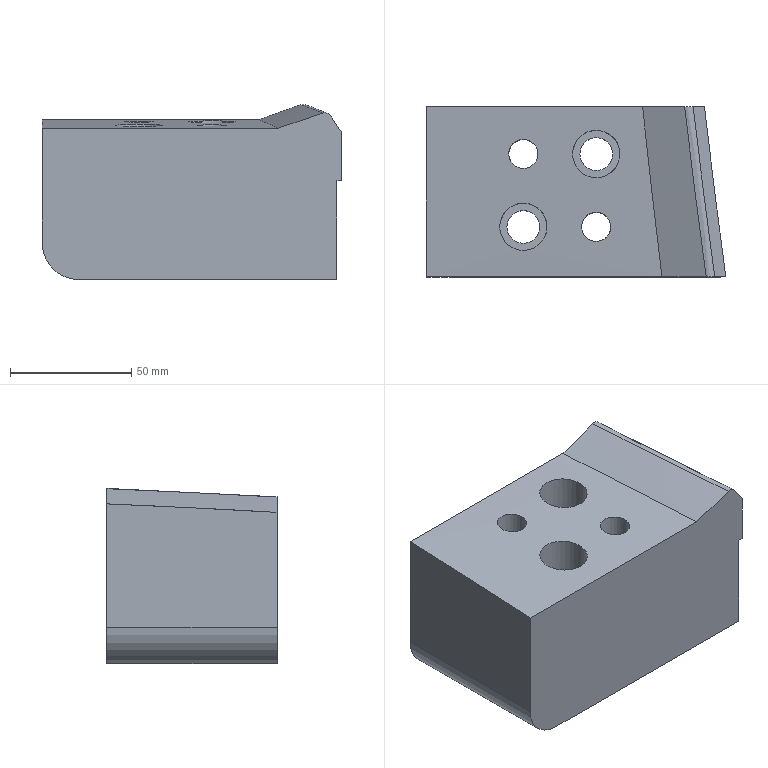Part | NX | features MAIN_BODY 2 | 1 solid | 20 faces | box 123.323 x 70 x 72.141 mm | volume 482943 mm3 | spline 7 | cylinder 7 | plane 6 | commonest cylinder face diameters 12 x2 13.5 x2 19.5 x2 30 x1
STEP:
#1=CARTESIAN_POINT('',(-841.75,-399.358,-100.));
#2=VERTEX_POINT('',#1);
#3=CARTESIAN_POINT('',(-835.,-399.358,-100.));
#4=DIRECTION('',(-0.000000341,0.00000017,-1.));
#5=DIRECTION('',(-1.,0.,0.000000341));
#6=AXIS2_PLACEMENT_3D('',#3,#4,#5);
#7=CIRCLE('',#6,6.75);
#8=EDGE_CURVE('',#2,#2,#7,.T.);
#9=ORIENTED_EDGE('',*,*,#8,.F.);
#10=EDGE_LOOP('',(#9));
#11=FACE_BOUND('',#10,.T.);
#12=CARTESIAN_POINT('',(-841.,-369.358,-100.));
#13=VERTEX_POINT('',#12);
#14=CARTESIAN_POINT('',(-835.,-369.358,-100.));
#15=DIRECTION('',(-0.000000341,0.00000017,-1.));
#16=DIRECTION('',(-1.,0.,0.000000341));
#17=AXIS2_PLACEMENT_3D('',#14,#15,#16);
#18=CIRCLE('',#17,6.);
#19=EDGE_CURVE('',#13,#13,#18,.T.);
#20=ORIENTED_EDGE('',*,*,#19,.F.);
#21=EDGE_LOOP('',(#20));
#22=FACE_BOUND('',#21,.T.);
#23=CARTESIAN_POINT('',(-811.75,-369.358,-100.));
#24=VERTEX_POINT('',#23);
#25=CARTESIAN_POINT('',(-805.,-369.358,-100.));
#26=DIRECTION('',(-0.000000341,0.00000017,-1.));
#27=DIRECTION('',(-1.,0.,0.000000341));
#28=AXIS2_PLACEMENT_3D('',#25,#26,#27);
#29=CIRCLE('',#28,6.75);
#30=EDGE_CURVE('',#24,#24,#29,.T.);
#31=ORIENTED_EDGE('',*,*,#30,.F.);
#32=EDGE_LOOP('',(#31));
#33=FACE_BOUND('',#32,.T.);
#34=CARTESIAN_POINT('',(-811.,-399.358,-100.));
#35=VERTEX_POINT('',#34);
#36=CARTESIAN_POINT('',(-805.,-399.358,-100.));
#37=DIRECTION('',(-0.000000341,0.00000017,-1.));
#38=DIRECTION('',(-1.,0.,0.000000341));
#39=AXIS2_PLACEMENT_3D('',#36,#37,#38);
#40=CIRCLE('',#39,6.);
#41=EDGE_CURVE('',#35,#35,#40,.T.);
#42=ORIENTED_EDGE('',*,*,#41,.F.);
#43=EDGE_LOOP('',(#42));
#44=FACE_BOUND('',#43,.T.);
#45=CARTESIAN_POINT('',(-860.,-350.,-100.));
#46=VERTEX_POINT('',#45);
#47=CARTESIAN_POINT('',(-762.48,-350.,-100.));
#48=VERTEX_POINT('',#47);
#49=CARTESIAN_POINT('',(-0.00003415,-350.,-100.));
#50=DIRECTION('',(-1.,0.,0.000000341));
#51=VECTOR('',#50,1000.);
#52=LINE('',#49,#51);
#53=EDGE_CURVE('',#46,#48,#52,.F.);
#54=ORIENTED_EDGE('',*,*,#53,.T.);
#55=CARTESIAN_POINT('',(-753.694,-420.,-100.));
#56=VERTEX_POINT('',#55);
#57=CARTESIAN_POINT('',(-753.694,-420.,-100.));
#58=CARTESIAN_POINT('',(-755.213,-408.34,-100.));
#59=CARTESIAN_POINT('',(-758.313,-385.028,-100.));
#60=CARTESIAN_POINT('',(-761.09,-361.676,-100.));
#61=CARTESIAN_POINT('',(-762.48,-350.,-100.));
#62=B_SPLINE_CURVE_WITH_KNOTS('',3,(#57,#58,#59,#60,#61),.UNSPECIFIED.,.F.,.F.,(4,1,4),(0.,0.03528,0.07055),.UNSPECIFIED.);
#63=EDGE_CURVE('',#56,#48,#62,.T.);
#64=ORIENTED_EDGE('',*,*,#63,.F.);
#65=CARTESIAN_POINT('',(-860.,-420.,-100.));
#66=VERTEX_POINT('',#65);
#67=CARTESIAN_POINT('',(-0.00003415,-420.,-100.));
#68=DIRECTION('',(-1.,0.,0.000000341));
#69=VECTOR('',#68,1000.);
#70=LINE('',#67,#69);
#71=EDGE_CURVE('',#66,#56,#70,.F.);
#72=ORIENTED_EDGE('',*,*,#71,.F.);
#73=CARTESIAN_POINT('',(-860.,-739.25,-100.));
#74=DIRECTION('',(0.000000011,1.,0.00000017));
#75=VECTOR('',#74,1000.);
#76=LINE('',#73,#75);
#77=EDGE_CURVE('',#46,#66,#76,.F.);
#78=ORIENTED_EDGE('',*,*,#77,.F.);
#79=EDGE_LOOP('',(#54,#64,#72,#78));
#80=FACE_BOUND('',#79,.T.);
#81=CARTESIAN_POINT('',(-780.,-1058.533,-100.));
#82=DIRECTION('',(-0.000000341,0.00000017,-1.));
#83=DIRECTION('',(-0.000000011,-1.,-0.00000017));
#84=AXIS2_PLACEMENT_3D('',#81,#82,#83);
#85=PLANE('',#84);
#86=ADVANCED_FACE('',(#11,#22,#33,#44,#80),#85,.T.);
#87=CARTESIAN_POINT('',(-751.677,-420.,-39.281));
#88=VERTEX_POINT('',#87);
#89=CARTESIAN_POINT('',(-756.237,-420.,-32.638));
#90=VERTEX_POINT('',#89);
#91=CARTESIAN_POINT('',(-751.677,-420.,-39.281));
#92=CARTESIAN_POINT('',(-753.197,-420.,-37.066));
#93=CARTESIAN_POINT('',(-754.717,-420.,-34.852));
#94=CARTESIAN_POINT('',(-756.237,-420.,-32.638));
#95=B_SPLINE_CURVE_WITH_KNOTS('',3,(#91,#92,#93,#94),.UNSPECIFIED.,.F.,.F.,(4,4),(0.,0.008057),.UNSPECIFIED.);
#96=EDGE_CURVE('',#88,#90,#95,.T.);
#97=ORIENTED_EDGE('',*,*,#96,.T.);
#98=CARTESIAN_POINT('',(-759.743,-420.,-31.477));
#99=VERTEX_POINT('',#98);
#100=CARTESIAN_POINT('',(-756.237,-420.,-32.638));
#101=CARTESIAN_POINT('',(-756.992,-420.,-31.539));
#102=CARTESIAN_POINT('',(-758.481,-420.,-31.044));
#103=CARTESIAN_POINT('',(-759.743,-420.,-31.477));
#104=B_SPLINE_CURVE_WITH_KNOTS('',3,(#100,#101,#102,#103),.UNSPECIFIED.,.F.,.F.,(4,4),(0.,0.003944),.UNSPECIFIED.);
#105=EDGE_CURVE('',#90,#99,#104,.T.);
#106=ORIENTED_EDGE('',*,*,#105,.T.);
#107=CARTESIAN_POINT('',(-777.971,-420.,-37.736));
#108=VERTEX_POINT('',#107);
#109=CARTESIAN_POINT('',(-759.743,-420.,-31.477));
#110=CARTESIAN_POINT('',(-765.819,-420.,-33.563));
#111=CARTESIAN_POINT('',(-771.895,-420.,-35.649));
#112=CARTESIAN_POINT('',(-777.971,-420.,-37.736));
#113=B_SPLINE_CURVE_WITH_KNOTS('',3,(#109,#110,#111,#112),.UNSPECIFIED.,.F.,.F.,(4,4),(0.,0.01927),.UNSPECIFIED.);
#114=EDGE_CURVE('',#99,#108,#113,.T.);
#115=ORIENTED_EDGE('',*,*,#114,.T.);
#116=CARTESIAN_POINT('',(-875.,-420.,-37.736));
#117=VERTEX_POINT('',#116);
#118=CARTESIAN_POINT('',(-875.,-420.,-37.736));
#119=CARTESIAN_POINT('',(-842.657,-420.,-37.736));
#120=CARTESIAN_POINT('',(-810.314,-420.,-37.736));
#121=CARTESIAN_POINT('',(-777.971,-420.,-37.736));
#122=B_SPLINE_CURVE_WITH_KNOTS('',3,(#118,#119,#120,#121),.UNSPECIFIED.,.F.,.F.,(4,4),(-0.01,0.08703),.UNSPECIFIED.);
#123=EDGE_CURVE('',#117,#108,#122,.T.);
#124=ORIENTED_EDGE('',*,*,#123,.F.);
#125=CARTESIAN_POINT('',(-875.,-420.,-85.));
#126=VERTEX_POINT('',#125);
#127=CARTESIAN_POINT('',(-875.,-420.,0.0002989));
#128=DIRECTION('',(0.000000341,0.,1.));
#129=VECTOR('',#128,1000.);
#130=LINE('',#127,#129);
#131=EDGE_CURVE('',#126,#117,#130,.T.);
#132=ORIENTED_EDGE('',*,*,#131,.F.);
#133=CARTESIAN_POINT('',(-860.,-420.,-85.));
#134=DIRECTION('',(0.,1.,0.));
#135=DIRECTION('',(0.,0.,1.));
#136=AXIS2_PLACEMENT_3D('',#133,#134,#135);
#137=CIRCLE('',#136,15.);
#138=EDGE_CURVE('',#66,#126,#137,.T.);
#139=ORIENTED_EDGE('',*,*,#138,.F.);
#140=ORIENTED_EDGE('',*,*,#71,.T.);
#141=CARTESIAN_POINT('',(-753.694,-420.,-59.267));
#142=VERTEX_POINT('',#141);
#143=CARTESIAN_POINT('',(-753.694,-420.,-74.594));
#144=DIRECTION('',(0.,0.,1.));
#145=VECTOR('',#144,1000.);
#146=LINE('',#143,#145);
#147=EDGE_CURVE('',#142,#56,#146,.F.);
#148=ORIENTED_EDGE('',*,*,#147,.F.);
#149=CARTESIAN_POINT('',(-751.677,-420.,-59.281));
#150=VERTEX_POINT('',#149);
#151=CARTESIAN_POINT('',(-753.694,-420.,-59.267));
#152=CARTESIAN_POINT('',(-753.022,-420.,-59.272));
#153=CARTESIAN_POINT('',(-752.35,-420.,-59.276));
#154=CARTESIAN_POINT('',(-751.677,-420.,-59.281));
#155=B_SPLINE_CURVE_WITH_KNOTS('',3,(#151,#152,#153,#154),.UNSPECIFIED.,.F.,.F.,(4,4),(0.,0.002017),.UNSPECIFIED.);
#156=EDGE_CURVE('',#142,#150,#155,.T.);
#157=ORIENTED_EDGE('',*,*,#156,.T.);
#158=CARTESIAN_POINT('',(-751.677,-420.,-49.201));
#159=DIRECTION('',(0.,0.,1.));
#160=VECTOR('',#159,1000.);
#161=LINE('',#158,#160);
#162=EDGE_CURVE('',#88,#150,#161,.F.);
#163=ORIENTED_EDGE('',*,*,#162,.F.);
#164=EDGE_LOOP('',(#97,#106,#115,#124,#132,#139,#140,#148,#157,#163));
#165=FACE_BOUND('',#164,.T.);
#166=CARTESIAN_POINT('',(0.,-420.,0.));
#167=DIRECTION('',(0.,1.,0.));
#168=DIRECTION('',(0.,0.,1.));
#169=AXIS2_PLACEMENT_3D('',#166,#167,#168);
#170=PLANE('',#169);
#171=ADVANCED_FACE('',(#165),#170,.F.);
#172=CARTESIAN_POINT('',(-760.466,-350.,-35.75));
#173=VERTEX_POINT('',#172);
#174=CARTESIAN_POINT('',(-760.466,-350.,-55.75));
#175=VERTEX_POINT('',#174);
#176=CARTESIAN_POINT('',(-760.466,-350.,-45.819));
#177=DIRECTION('',(0.,0.,1.));
#178=VECTOR('',#177,1000.);
#179=LINE('',#176,#178);
#180=EDGE_CURVE('',#173,#175,#179,.F.);
#181=ORIENTED_EDGE('',*,*,#180,.F.);
#182=CARTESIAN_POINT('',(-760.466,-350.,-35.75));
#183=CARTESIAN_POINT('',(-759.076,-361.679,-36.278));
#184=CARTESIAN_POINT('',(-756.296,-385.037,-37.348));
#185=CARTESIAN_POINT('',(-753.196,-408.342,-38.648));
#186=CARTESIAN_POINT('',(-751.677,-420.,-39.281));
#187=B_SPLINE_CURVE_WITH_KNOTS('',3,(#182,#183,#184,#185,#186),.UNSPECIFIED.,.F.,.F.,(4,1,4),(-0.001545,0.03377,0.06909),.UNSPECIFIED.);
#188=EDGE_CURVE('',#173,#88,#187,.T.);
#189=ORIENTED_EDGE('',*,*,#188,.T.);
#190=ORIENTED_EDGE('',*,*,#162,.T.);
#191=CARTESIAN_POINT('',(-751.677,-420.,-59.281));
#192=CARTESIAN_POINT('',(-753.196,-408.342,-58.648));
#193=CARTESIAN_POINT('',(-756.296,-385.037,-57.348));
#194=CARTESIAN_POINT('',(-759.076,-361.679,-56.278));
#195=CARTESIAN_POINT('',(-760.466,-350.,-55.75));
#196=B_SPLINE_CURVE_WITH_KNOTS('',3,(#191,#192,#193,#194,#195),.UNSPECIFIED.,.F.,.F.,(4,1,4),(-0.001482,0.03384,0.06916),.UNSPECIFIED.);
#197=EDGE_CURVE('',#150,#175,#196,.T.);
#198=ORIENTED_EDGE('',*,*,#197,.T.);
#199=EDGE_LOOP('',(#181,#189,#190,#198));
#200=FACE_BOUND('',#199,.T.);
#201=CARTESIAN_POINT('',(-760.466,-350.,-55.89));
#202=CARTESIAN_POINT('',(-760.466,-350.,-35.604));
#203=CARTESIAN_POINT('',(-759.076,-361.678,-56.437));
#204=CARTESIAN_POINT('',(-759.076,-361.678,-36.15));
#205=CARTESIAN_POINT('',(-756.296,-385.034,-57.531));
#206=CARTESIAN_POINT('',(-756.296,-385.034,-37.244));
#207=CARTESIAN_POINT('',(-753.196,-408.342,-58.788));
#208=CARTESIAN_POINT('',(-753.196,-408.342,-38.501));
#209=CARTESIAN_POINT('',(-751.677,-420.,-59.401));
#210=CARTESIAN_POINT('',(-751.677,-420.,-39.114));
#211=B_SPLINE_SURFACE_WITH_KNOTS('',3,1,((#201,#202),(#203,#204),(#205,#206),(#207,#208),(#209,#210)),.SURF_OF_LINEAR_EXTRUSION.,.F.,.F.,.F.,(4,1,4),(2,2),(-0.4271,0.68,1.787),(0.,1.),.UNSPECIFIED.);
#212=ADVANCED_FACE('',(#200),#211,.F.);
#213=ORIENTED_EDGE('',*,*,#131,.T.);
#214=CARTESIAN_POINT('',(-875.,-350.,-34.252));
#215=VERTEX_POINT('',#214);
#216=CARTESIAN_POINT('',(-875.,-350.,-34.252));
#217=CARTESIAN_POINT('',(-875.,-373.342,-35.241));
#218=CARTESIAN_POINT('',(-875.,-396.676,-36.394));
#219=CARTESIAN_POINT('',(-875.,-420.,-37.736));
#220=B_SPLINE_CURVE_WITH_KNOTS('',3,(#216,#217,#218,#219),.UNSPECIFIED.,.F.,.F.,(4,4),(0.2837,0.3538),.UNSPECIFIED.);
#221=EDGE_CURVE('',#117,#215,#220,.F.);
#222=ORIENTED_EDGE('',*,*,#221,.T.);
#223=CARTESIAN_POINT('',(-875.,-350.,-85.));
#224=VERTEX_POINT('',#223);
#225=CARTESIAN_POINT('',(-875.,-350.,0.0002989));
#226=DIRECTION('',(0.000000341,0.,1.));
#227=VECTOR('',#226,1000.);
#228=LINE('',#225,#227);
#229=EDGE_CURVE('',#224,#215,#228,.T.);
#230=ORIENTED_EDGE('',*,*,#229,.F.);
#231=CARTESIAN_POINT('',(-875.,-739.25,-85.));
#232=DIRECTION('',(0.000000011,1.,0.00000017));
#233=VECTOR('',#232,1000.);
#234=LINE('',#231,#233);
#235=EDGE_CURVE('',#126,#224,#234,.T.);
#236=ORIENTED_EDGE('',*,*,#235,.F.);
#237=EDGE_LOOP('',(#213,#222,#230,#236));
#238=FACE_BOUND('',#237,.T.);
#239=CARTESIAN_POINT('',(-875.,-739.25,-90.));
#240=DIRECTION('',(-1.,0.000000011,0.000000341));
#241=DIRECTION('',(-0.000000341,0.00000017,-1.));
#242=AXIS2_PLACEMENT_3D('',#239,#240,#241);
#243=PLANE('',#242);
#244=ADVANCED_FACE('',(#238),#243,.T.);
#245=CARTESIAN_POINT('',(-802.615,-378.812,-35.56));
#246=VERTEX_POINT('',#245);
#247=CARTESIAN_POINT('',(-810.554,-378.63,-35.551));
#248=CARTESIAN_POINT('',(-802.353,-379.838,-35.61));
#249=CARTESIAN_POINT('',(-795.722,-374.891,-35.371));
#250=CARTESIAN_POINT('',(-794.523,-366.727,-34.987));
#251=CARTESIAN_POINT('',(-799.45,-360.085,-34.688));
#252=CARTESIAN_POINT('',(-807.643,-358.881,-34.635));
#253=CARTESIAN_POINT('',(-814.27,-363.813,-34.854));
#254=CARTESIAN_POINT('',(-815.479,-371.987,-35.232));
#255=CARTESIAN_POINT('',(-810.554,-378.63,-35.551));
#256=CARTESIAN_POINT('',(-802.353,-379.838,-35.61));
#257=CARTESIAN_POINT('',(-795.722,-374.891,-35.371));
#258=B_SPLINE_CURVE_WITH_KNOTS('',3,(#247,#248,#249,#250,#251,#252,#253,#254,#255,#256,#257),.UNSPECIFIED.,.T.,.F.,(1,1,1,1,1,1,1,1,1,1,1,1,1,1,1),(-0.02287,-0.01525,-0.007624,0.,0.007624,0.01525,0.02287,0.0305,0.03812,0.04574,0.05337,0.06099,0.06862,0.07624,0.08386),.UNSPECIFIED.);
#259=EDGE_CURVE('',#246,#246,#258,.T.);
#260=ORIENTED_EDGE('',*,*,#259,.F.);
#261=EDGE_LOOP('',(#260));
#262=FACE_BOUND('',#261,.T.);
#263=CARTESIAN_POINT('',(-806.104,-405.256,-36.91));
#264=VERTEX_POINT('',#263);
#265=CARTESIAN_POINT('',(-810.492,-403.108,-36.793));
#266=CARTESIAN_POINT('',(-806.223,-405.897,-36.944));
#267=CARTESIAN_POINT('',(-801.239,-404.841,-36.887));
#268=CARTESIAN_POINT('',(-798.467,-400.584,-36.658));
#269=CARTESIAN_POINT('',(-799.51,-395.607,-36.398));
#270=CARTESIAN_POINT('',(-803.775,-392.823,-36.256));
#271=CARTESIAN_POINT('',(-808.753,-393.871,-36.309));
#272=CARTESIAN_POINT('',(-811.534,-398.131,-36.529));
#273=CARTESIAN_POINT('',(-810.492,-403.108,-36.793));
#274=CARTESIAN_POINT('',(-806.223,-405.897,-36.944));
#275=CARTESIAN_POINT('',(-801.239,-404.841,-36.887));
#276=B_SPLINE_CURVE_WITH_KNOTS('',3,(#265,#266,#267,#268,#269,#270,#271,#272,#273,#274,#275),.UNSPECIFIED.,.T.,.F.,(1,1,1,1,1,1,1,1,1,1,1,1,1,1,1),(-0.01408,-0.009385,-0.004692,0.,0.004692,0.009385,0.01408,0.01877,0.02346,0.02815,0.03285,0.03754,0.04223,0.04692,0.05162),.UNSPECIFIED.);
#277=EDGE_CURVE('',#264,#264,#276,.T.);
#278=ORIENTED_EDGE('',*,*,#277,.F.);
#279=EDGE_LOOP('',(#278));
#280=FACE_BOUND('',#279,.T.);
#281=CARTESIAN_POINT('',(-785.933,-350.,-34.252));
#282=VERTEX_POINT('',#281);
#283=CARTESIAN_POINT('',(-875.,-350.,-34.252));
#284=CARTESIAN_POINT('',(-845.311,-350.,-34.252));
#285=CARTESIAN_POINT('',(-815.622,-350.,-34.252));
#286=CARTESIAN_POINT('',(-785.933,-350.,-34.252));
#287=B_SPLINE_CURVE_WITH_KNOTS('',3,(#283,#284,#285,#286),.UNSPECIFIED.,.F.,.F.,(4,4),(-0.01,0.07907),.UNSPECIFIED.);
#288=EDGE_CURVE('',#215,#282,#287,.T.);
#289=ORIENTED_EDGE('',*,*,#288,.F.);
#290=ORIENTED_EDGE('',*,*,#221,.F.);
#291=ORIENTED_EDGE('',*,*,#123,.T.);
#292=CARTESIAN_POINT('',(-777.971,-420.,-37.736));
#293=CARTESIAN_POINT('',(-780.789,-396.695,-36.395));
#294=CARTESIAN_POINT('',(-783.443,-373.36,-35.242));
#295=CARTESIAN_POINT('',(-785.933,-350.,-34.252));
#296=B_SPLINE_CURVE_WITH_KNOTS('',3,(#292,#293,#294,#295),.UNSPECIFIED.,.F.,.F.,(4,4),(0.1656,0.2359),.UNSPECIFIED.);
#297=EDGE_CURVE('',#108,#282,#296,.T.);
#298=ORIENTED_EDGE('',*,*,#297,.T.);
#299=EDGE_LOOP('',(#289,#290,#291,#298));
#300=FACE_BOUND('',#299,.T.);
#301=CARTESIAN_POINT('',(-837.117,-374.973,-35.376));
#302=VERTEX_POINT('',#301);
#303=CARTESIAN_POINT('',(-841.061,-372.092,-35.239));
#304=CARTESIAN_POINT('',(-837.346,-375.582,-35.405));
#305=CARTESIAN_POINT('',(-832.255,-375.414,-35.397));
#306=CARTESIAN_POINT('',(-828.781,-371.706,-35.22));
#307=CARTESIAN_POINT('',(-828.94,-366.622,-34.983));
#308=CARTESIAN_POINT('',(-832.652,-363.137,-34.825));
#309=CARTESIAN_POINT('',(-837.736,-363.299,-34.832));
#310=CARTESIAN_POINT('',(-841.22,-367.009,-35.001));
#311=CARTESIAN_POINT('',(-841.061,-372.092,-35.239));
#312=CARTESIAN_POINT('',(-837.346,-375.582,-35.405));
#313=CARTESIAN_POINT('',(-832.255,-375.414,-35.397));
#314=B_SPLINE_CURVE_WITH_KNOTS('',3,(#303,#304,#305,#306,#307,#308,#309,#310,#311,#312,#313),.UNSPECIFIED.,.T.,.F.,(1,1,1,1,1,1,1,1,1,1,1,1,1,1,1),(-0.01408,-0.009384,-0.004692,0.,0.004692,0.009384,0.01408,0.01877,0.02346,0.02815,0.03284,0.03753,0.04223,0.04692,0.05161),.UNSPECIFIED.);
#315=EDGE_CURVE('',#302,#302,#314,.T.);
#316=ORIENTED_EDGE('',*,*,#315,.F.);
#317=EDGE_LOOP('',(#316));
#318=FACE_BOUND('',#317,.T.);
#319=CARTESIAN_POINT('',(-844.701,-400.333,-36.646));
#320=VERTEX_POINT('',#319);
#321=CARTESIAN_POINT('',(-843.364,-392.516,-36.238));
#322=CARTESIAN_POINT('',(-845.751,-400.44,-36.648));
#323=CARTESIAN_POINT('',(-841.839,-407.721,-37.043));
#324=CARTESIAN_POINT('',(-833.927,-410.11,-37.176));
#325=CARTESIAN_POINT('',(-826.634,-406.198,-36.959));
#326=CARTESIAN_POINT('',(-824.252,-398.282,-36.535));
#327=CARTESIAN_POINT('',(-828.148,-391.005,-36.162));
#328=CARTESIAN_POINT('',(-836.069,-388.604,-36.043));
#329=CARTESIAN_POINT('',(-843.364,-392.516,-36.238));
#330=CARTESIAN_POINT('',(-845.751,-400.44,-36.648));
#331=CARTESIAN_POINT('',(-841.839,-407.721,-37.043));
#332=B_SPLINE_CURVE_WITH_KNOTS('',3,(#321,#322,#323,#324,#325,#326,#327,#328,#329,#330,#331),.UNSPECIFIED.,.T.,.F.,(1,1,1,1,1,1,1,1,1,1,1,1,1,1,1),(-0.02288,-0.01525,-0.007625,0.,0.007625,0.01525,0.02288,0.0305,0.03813,0.04575,0.05338,0.061,0.06863,0.07625,0.08388),.UNSPECIFIED.);
#333=EDGE_CURVE('',#320,#320,#332,.T.);
#334=ORIENTED_EDGE('',*,*,#333,.F.);
#335=EDGE_LOOP('',(#334));
#336=FACE_BOUND('',#335,.T.);
#337=CARTESIAN_POINT('',(-875.566,-420.159,-37.746));
#338=CARTESIAN_POINT('',(-776.547,-420.159,-37.746));
#339=CARTESIAN_POINT('',(-877.1,-408.39,-37.068));
#340=CARTESIAN_POINT('',(-778.081,-408.39,-37.068));
#341=CARTESIAN_POINT('',(-880.224,-384.914,-35.815));
#342=CARTESIAN_POINT('',(-781.205,-384.914,-35.815));
#343=CARTESIAN_POINT('',(-883.011,-361.373,-34.734));
#344=CARTESIAN_POINT('',(-783.992,-361.373,-34.734));
#345=CARTESIAN_POINT('',(-884.415,-349.579,-34.234));
#346=CARTESIAN_POINT('',(-785.396,-349.579,-34.234));
#347=B_SPLINE_SURFACE_WITH_KNOTS('',3,1,((#337,#338),(#339,#340),(#341,#342),(#343,#344),(#345,#346)),.SURF_OF_LINEAR_EXTRUSION.,.F.,.F.,.F.,(4,1,4),(2,2),(-0.0303,0.4972,1.025),(0.,1.),.UNSPECIFIED.);
#348=ADVANCED_FACE('',(#262,#280,#300,#318,#336),#347,.F.);
#349=CARTESIAN_POINT('',(-768.637,-350.,-28.029));
#350=VERTEX_POINT('',#349);
#351=CARTESIAN_POINT('',(-768.637,-350.,-28.029));
#352=CARTESIAN_POINT('',(-774.403,-350.,-30.103));
#353=CARTESIAN_POINT('',(-780.168,-350.,-32.177));
#354=CARTESIAN_POINT('',(-785.933,-350.,-34.252));
#355=B_SPLINE_CURVE_WITH_KNOTS('',3,(#351,#352,#353,#354),.UNSPECIFIED.,.F.,.F.,(4,4),(0.,0.01838),.UNSPECIFIED.);
#356=EDGE_CURVE('',#350,#282,#355,.T.);
#357=ORIENTED_EDGE('',*,*,#356,.F.);
#358=CARTESIAN_POINT('',(-765.126,-350.,-29.138));
#359=VERTEX_POINT('',#358);
#360=CARTESIAN_POINT('',(-768.637,-350.,-28.029));
#361=CARTESIAN_POINT('',(-767.385,-350.,-27.578));
#362=CARTESIAN_POINT('',(-765.892,-350.,-28.05));
#363=CARTESIAN_POINT('',(-765.126,-350.,-29.138));
#364=B_SPLINE_CURVE_WITH_KNOTS('',3,(#360,#361,#362,#363),.UNSPECIFIED.,.F.,.F.,(4,4),(0.,0.003934),.UNSPECIFIED.);
#365=EDGE_CURVE('',#350,#359,#364,.T.);
#366=ORIENTED_EDGE('',*,*,#365,.T.);
#367=CARTESIAN_POINT('',(-765.126,-350.,-29.138));
#368=CARTESIAN_POINT('',(-763.572,-350.,-31.342));
#369=CARTESIAN_POINT('',(-762.019,-350.,-33.546));
#370=CARTESIAN_POINT('',(-760.466,-350.,-35.75));
#371=B_SPLINE_CURVE_WITH_KNOTS('',3,(#367,#368,#369,#370),.UNSPECIFIED.,.F.,.F.,(4,4),(0.,0.008089),.UNSPECIFIED.);
#372=EDGE_CURVE('',#359,#173,#371,.T.);
#373=ORIENTED_EDGE('',*,*,#372,.T.);
#374=ORIENTED_EDGE('',*,*,#180,.T.);
#375=CARTESIAN_POINT('',(-762.48,-350.,-55.739));
#376=VERTEX_POINT('',#375);
#377=CARTESIAN_POINT('',(-760.466,-350.,-55.75));
#378=CARTESIAN_POINT('',(-761.137,-350.,-55.746));
#379=CARTESIAN_POINT('',(-761.808,-350.,-55.743));
#380=CARTESIAN_POINT('',(-762.48,-350.,-55.739));
#381=B_SPLINE_CURVE_WITH_KNOTS('',3,(#377,#378,#379,#380),.UNSPECIFIED.,.F.,.F.,(4,4),(0.,0.002014),.UNSPECIFIED.);
#382=EDGE_CURVE('',#175,#376,#381,.T.);
#383=ORIENTED_EDGE('',*,*,#382,.T.);
#384=CARTESIAN_POINT('',(-762.48,-350.,-72.904));
#385=DIRECTION('',(0.,0.,1.));
#386=VECTOR('',#385,1000.);
#387=LINE('',#384,#386);
#388=EDGE_CURVE('',#376,#48,#387,.F.);
#389=ORIENTED_EDGE('',*,*,#388,.T.);
#390=ORIENTED_EDGE('',*,*,#53,.F.);
#391=CARTESIAN_POINT('',(-860.,-350.,-85.));
#392=DIRECTION('',(0.,1.,0.));
#393=DIRECTION('',(0.,0.,1.));
#394=AXIS2_PLACEMENT_3D('',#391,#392,#393);
#395=CIRCLE('',#394,15.);
#396=EDGE_CURVE('',#224,#46,#395,.F.);
#397=ORIENTED_EDGE('',*,*,#396,.F.);
#398=ORIENTED_EDGE('',*,*,#229,.T.);
#399=ORIENTED_EDGE('',*,*,#288,.T.);
#400=EDGE_LOOP('',(#357,#366,#373,#374,#383,#389,#390,#397,#398,#399));
#401=FACE_BOUND('',#400,.T.);
#402=CARTESIAN_POINT('',(0.,-350.,0.));
#403=DIRECTION('',(0.,1.,0.));
#404=DIRECTION('',(0.,0.,1.));
#405=AXIS2_PLACEMENT_3D('',#402,#403,#404);
#406=PLANE('',#405);
#407=ADVANCED_FACE('',(#401),#406,.T.);
#408=CARTESIAN_POINT('',(-844.75,-399.358,-80.));
#409=VERTEX_POINT('',#408);
#410=CARTESIAN_POINT('',(-835.,-399.358,-80.));
#411=DIRECTION('',(0.000000341,-0.00000017,1.));
#412=DIRECTION('',(-1.,0.,0.000000341));
#413=AXIS2_PLACEMENT_3D('',#410,#411,#412);
#414=CIRCLE('',#413,9.75);
#415=EDGE_CURVE('',#409,#409,#414,.F.);
#416=ORIENTED_EDGE('',*,*,#415,.T.);
#417=EDGE_LOOP('',(#416));
#418=FACE_BOUND('',#417,.T.);
#419=ORIENTED_EDGE('',*,*,#333,.T.);
#420=EDGE_LOOP('',(#419));
#421=FACE_BOUND('',#420,.T.);
#422=CARTESIAN_POINT('',(-835.,-399.358,-70.));
#423=DIRECTION('',(0.000000341,-0.00000017,1.));
#424=DIRECTION('',(0.000000011,1.,0.00000017));
#425=AXIS2_PLACEMENT_3D('',#422,#423,#424);
#426=CYLINDRICAL_SURFACE('',#425,9.75);
#427=ADVANCED_FACE('',(#418,#421),#426,.F.);
#428=CARTESIAN_POINT('',(-841.75,-399.358,-80.));
#429=VERTEX_POINT('',#428);
#430=CARTESIAN_POINT('',(-835.,-399.358,-80.));
#431=DIRECTION('',(0.000000341,-0.00000017,1.));
#432=DIRECTION('',(-1.,0.,0.000000341));
#433=AXIS2_PLACEMENT_3D('',#430,#431,#432);
#434=CIRCLE('',#433,6.75);
#435=EDGE_CURVE('',#429,#429,#434,.F.);
#436=ORIENTED_EDGE('',*,*,#435,.F.);
#437=EDGE_LOOP('',(#436));
#438=FACE_BOUND('',#437,.T.);
#439=ORIENTED_EDGE('',*,*,#8,.T.);
#440=EDGE_LOOP('',(#439));
#441=FACE_BOUND('',#440,.T.);
#442=CARTESIAN_POINT('',(-835.,-399.358,-90.));
#443=DIRECTION('',(0.000000341,-0.00000017,1.));
#444=DIRECTION('',(0.000000011,1.,0.00000017));
#445=AXIS2_PLACEMENT_3D('',#442,#443,#444);
#446=CYLINDRICAL_SURFACE('',#445,6.75);
#447=ADVANCED_FACE('',(#438,#441),#446,.F.);
#448=ORIENTED_EDGE('',*,*,#435,.T.);
#449=EDGE_LOOP('',(#448));
#450=FACE_BOUND('',#449,.T.);
#451=ORIENTED_EDGE('',*,*,#415,.F.);
#452=EDGE_LOOP('',(#451));
#453=FACE_BOUND('',#452,.T.);
#454=CARTESIAN_POINT('',(-835.,-399.358,-80.));
#455=DIRECTION('',(-0.000000341,0.00000017,-1.));
#456=DIRECTION('',(-0.000000011,-1.,-0.00000017));
#457=AXIS2_PLACEMENT_3D('',#454,#455,#456);
#458=PLANE('',#457);
#459=ADVANCED_FACE('',(#450,#453),#458,.F.);
#460=ORIENTED_EDGE('',*,*,#19,.T.);
#461=EDGE_LOOP('',(#460));
#462=FACE_BOUND('',#461,.T.);
#463=ORIENTED_EDGE('',*,*,#315,.T.);
#464=EDGE_LOOP('',(#463));
#465=FACE_BOUND('',#464,.T.);
#466=CARTESIAN_POINT('',(-835.,-369.358,-90.));
#467=DIRECTION('',(0.000000341,-0.00000017,1.));
#468=DIRECTION('',(0.000000011,1.,0.00000017));
#469=AXIS2_PLACEMENT_3D('',#466,#467,#468);
#470=CYLINDRICAL_SURFACE('',#469,6.);
#471=ADVANCED_FACE('',(#462,#465),#470,.F.);
#472=CARTESIAN_POINT('',(-814.75,-369.358,-80.));
#473=VERTEX_POINT('',#472);
#474=CARTESIAN_POINT('',(-805.,-369.358,-80.));
#475=DIRECTION('',(0.000000341,-0.00000017,1.));
#476=DIRECTION('',(-1.,0.,0.000000341));
#477=AXIS2_PLACEMENT_3D('',#474,#475,#476);
#478=CIRCLE('',#477,9.75);
#479=EDGE_CURVE('',#473,#473,#478,.F.);
#480=ORIENTED_EDGE('',*,*,#479,.T.);
#481=EDGE_LOOP('',(#480));
#482=FACE_BOUND('',#481,.T.);
#483=ORIENTED_EDGE('',*,*,#259,.T.);
#484=EDGE_LOOP('',(#483));
#485=FACE_BOUND('',#484,.T.);
#486=CARTESIAN_POINT('',(-805.,-369.358,-70.));
#487=DIRECTION('',(0.000000341,-0.00000017,1.));
#488=DIRECTION('',(0.000000011,1.,0.00000017));
#489=AXIS2_PLACEMENT_3D('',#486,#487,#488);
#490=CYLINDRICAL_SURFACE('',#489,9.75);
#491=ADVANCED_FACE('',(#482,#485),#490,.F.);
#492=CARTESIAN_POINT('',(-811.75,-369.358,-80.));
#493=VERTEX_POINT('',#492);
#494=CARTESIAN_POINT('',(-805.,-369.358,-80.));
#495=DIRECTION('',(0.000000341,-0.00000017,1.));
#496=DIRECTION('',(-1.,0.,0.000000341));
#497=AXIS2_PLACEMENT_3D('',#494,#495,#496);
#498=CIRCLE('',#497,6.75);
#499=EDGE_CURVE('',#493,#493,#498,.F.);
#500=ORIENTED_EDGE('',*,*,#499,.F.);
#501=EDGE_LOOP('',(#500));
#502=FACE_BOUND('',#501,.T.);
#503=ORIENTED_EDGE('',*,*,#30,.T.);
#504=EDGE_LOOP('',(#503));
#505=FACE_BOUND('',#504,.T.);
#506=CARTESIAN_POINT('',(-805.,-369.358,-90.));
#507=DIRECTION('',(0.000000341,-0.00000017,1.));
#508=DIRECTION('',(0.000000011,1.,0.00000017));
#509=AXIS2_PLACEMENT_3D('',#506,#507,#508);
#510=CYLINDRICAL_SURFACE('',#509,6.75);
#511=ADVANCED_FACE('',(#502,#505),#510,.F.);
#512=ORIENTED_EDGE('',*,*,#499,.T.);
#513=EDGE_LOOP('',(#512));
#514=FACE_BOUND('',#513,.T.);
#515=ORIENTED_EDGE('',*,*,#479,.F.);
#516=EDGE_LOOP('',(#515));
#517=FACE_BOUND('',#516,.T.);
#518=CARTESIAN_POINT('',(-805.,-369.358,-80.));
#519=DIRECTION('',(-0.000000341,0.00000017,-1.));
#520=DIRECTION('',(-0.000000011,-1.,-0.00000017));
#521=AXIS2_PLACEMENT_3D('',#518,#519,#520);
#522=PLANE('',#521);
#523=ADVANCED_FACE('',(#514,#517),#522,.F.);
#524=ORIENTED_EDGE('',*,*,#41,.T.);
#525=EDGE_LOOP('',(#524));
#526=FACE_BOUND('',#525,.T.);
#527=ORIENTED_EDGE('',*,*,#277,.T.);
#528=EDGE_LOOP('',(#527));
#529=FACE_BOUND('',#528,.T.);
#530=CARTESIAN_POINT('',(-805.,-399.358,-90.));
#531=DIRECTION('',(0.000000341,-0.00000017,1.));
#532=DIRECTION('',(0.000000011,1.,0.00000017));
#533=AXIS2_PLACEMENT_3D('',#530,#531,#532);
#534=CYLINDRICAL_SURFACE('',#533,6.);
#535=ADVANCED_FACE('',(#526,#529),#534,.F.);
#536=ORIENTED_EDGE('',*,*,#156,.F.);
#537=CARTESIAN_POINT('',(-753.694,-420.,-59.267));
#538=CARTESIAN_POINT('',(-755.213,-408.342,-58.634));
#539=CARTESIAN_POINT('',(-758.312,-385.037,-57.335));
#540=CARTESIAN_POINT('',(-761.09,-361.679,-56.267));
#541=CARTESIAN_POINT('',(-762.48,-350.,-55.739));
#542=B_SPLINE_CURVE_WITH_KNOTS('',3,(#537,#538,#539,#540,#541),.UNSPECIFIED.,.F.,.F.,(4,1,4),(-0.001482,0.03384,0.06916),.UNSPECIFIED.);
#543=EDGE_CURVE('',#142,#376,#542,.T.);
#544=ORIENTED_EDGE('',*,*,#543,.T.);
#545=ORIENTED_EDGE('',*,*,#382,.F.);
#546=ORIENTED_EDGE('',*,*,#197,.F.);
#547=EDGE_LOOP('',(#536,#544,#545,#546));
#548=FACE_BOUND('',#547,.T.);
#549=CARTESIAN_POINT('',(-751.658,-419.997,-59.281));
#550=CARTESIAN_POINT('',(-751.721,-419.508,-59.254));
#551=CARTESIAN_POINT('',(-751.785,-419.019,-59.228));
#552=CARTESIAN_POINT('',(-751.849,-418.53,-59.201));
#553=CARTESIAN_POINT('',(-753.303,-407.372,-58.596));
#554=CARTESIAN_POINT('',(-754.778,-396.218,-57.973));
#555=CARTESIAN_POINT('',(-757.606,-373.887,-56.841));
#556=CARTESIAN_POINT('',(-758.933,-362.709,-56.325));
#557=CARTESIAN_POINT('',(-760.264,-351.53,-55.819));
#558=CARTESIAN_POINT('',(-760.29,-351.307,-55.809));
#559=CARTESIAN_POINT('',(-760.317,-351.083,-55.799));
#560=CARTESIAN_POINT('',(-760.343,-350.86,-55.789));
#561=CARTESIAN_POINT('',(-760.387,-350.493,-55.772));
#562=CARTESIAN_POINT('',(-760.431,-350.127,-55.756));
#563=CARTESIAN_POINT('',(-760.474,-349.761,-55.739));
#564=CARTESIAN_POINT('',(-753.678,-420.261,-59.281));
#565=CARTESIAN_POINT('',(-753.742,-419.771,-59.254));
#566=CARTESIAN_POINT('',(-753.806,-419.282,-59.228));
#567=CARTESIAN_POINT('',(-753.869,-418.793,-59.201));
#568=CARTESIAN_POINT('',(-755.323,-407.637,-58.596));
#569=CARTESIAN_POINT('',(-756.799,-396.482,-57.973));
#570=CARTESIAN_POINT('',(-759.629,-374.135,-56.841));
#571=CARTESIAN_POINT('',(-760.957,-362.946,-56.325));
#572=CARTESIAN_POINT('',(-762.287,-351.771,-55.819));
#573=CARTESIAN_POINT('',(-762.313,-351.548,-55.809));
#574=CARTESIAN_POINT('',(-762.34,-351.324,-55.799));
#575=CARTESIAN_POINT('',(-762.367,-351.101,-55.789));
#576=CARTESIAN_POINT('',(-762.41,-350.734,-55.772));
#577=CARTESIAN_POINT('',(-762.454,-350.368,-55.756));
#578=CARTESIAN_POINT('',(-762.497,-350.002,-55.739));
#579=B_SPLINE_SURFACE_WITH_KNOTS('',1,3,((#549,#550,#551,#552,#553,#554,#555,#556,#557,#558,#559,#560,#561,#562,#563),(#564,#565,#566,#567,#568,#569,#570,#571,#572,#573,#574,#575,#576,#577,#578)),.RULED_SURF.,.F.,.F.,.F.,(2,2),(4,3,2,3,3,4),(0.498,0.7018),(-0.02192,0.,0.5,1.,1.01,1.026),.UNSPECIFIED.);
#580=ADVANCED_FACE('',(#548),#579,.T.);
#581=ORIENTED_EDGE('',*,*,#543,.F.);
#582=ORIENTED_EDGE('',*,*,#147,.T.);
#583=ORIENTED_EDGE('',*,*,#63,.T.);
#584=ORIENTED_EDGE('',*,*,#388,.F.);
#585=EDGE_LOOP('',(#581,#582,#583,#584));
#586=FACE_BOUND('',#585,.T.);
#587=CARTESIAN_POINT('',(-762.48,-350.,-100.266));
#588=CARTESIAN_POINT('',(-762.48,-350.,-55.446));
#589=CARTESIAN_POINT('',(-761.09,-361.674,-100.812));
#590=CARTESIAN_POINT('',(-761.09,-361.674,-55.993));
#591=CARTESIAN_POINT('',(-758.311,-385.042,-101.904));
#592=CARTESIAN_POINT('',(-758.311,-385.042,-57.085));
#593=CARTESIAN_POINT('',(-755.213,-408.345,-103.161));
#594=CARTESIAN_POINT('',(-755.213,-408.345,-58.342));
#595=CARTESIAN_POINT('',(-753.694,-420.,-103.774));
#596=CARTESIAN_POINT('',(-753.694,-420.,-58.954));
#597=B_SPLINE_SURFACE_WITH_KNOTS('',3,1,((#587,#588),(#589,#590),(#591,#592),(#593,#594),(#595,#596)),.SURF_OF_LINEAR_EXTRUSION.,.F.,.F.,.F.,(4,1,4),(2,2),(-0.4346,0.6722,1.779),(0.,1.),.UNSPECIFIED.);
#598=ADVANCED_FACE('',(#586),#597,.F.);
#599=ORIENTED_EDGE('',*,*,#138,.T.);
#600=ORIENTED_EDGE('',*,*,#235,.T.);
#601=ORIENTED_EDGE('',*,*,#396,.T.);
#602=ORIENTED_EDGE('',*,*,#77,.T.);
#603=EDGE_LOOP('',(#599,#600,#601,#602));
#604=FACE_BOUND('',#603,.T.);
#605=CARTESIAN_POINT('',(-860.,-739.25,-85.));
#606=DIRECTION('',(0.000000011,1.,0.00000017));
#607=DIRECTION('',(-0.000000341,0.00000017,-1.));
#608=AXIS2_PLACEMENT_3D('',#605,#606,#607);
#609=CYLINDRICAL_SURFACE('',#608,15.);
#610=ADVANCED_FACE('',(#604),#609,.T.);
#611=ORIENTED_EDGE('',*,*,#114,.F.);
#612=CARTESIAN_POINT('',(-759.743,-420.,-31.477));
#613=CARTESIAN_POINT('',(-762.888,-396.7,-30.139));
#614=CARTESIAN_POINT('',(-765.861,-373.365,-29.002));
#615=CARTESIAN_POINT('',(-768.637,-350.,-28.029));
#616=B_SPLINE_CURVE_WITH_KNOTS('',3,(#612,#613,#614,#615),.UNSPECIFIED.,.F.,.F.,(4,4),(-0.001483,0.06917),.UNSPECIFIED.);
#617=EDGE_CURVE('',#99,#350,#616,.T.);
#618=ORIENTED_EDGE('',*,*,#617,.T.);
#619=ORIENTED_EDGE('',*,*,#356,.T.);
#620=ORIENTED_EDGE('',*,*,#297,.F.);
#621=EDGE_LOOP('',(#611,#618,#619,#620));
#622=FACE_BOUND('',#621,.T.);
#623=CARTESIAN_POINT('',(-786.407,-349.588,-34.389));
#624=CARTESIAN_POINT('',(-780.371,-349.42,-32.203));
#625=CARTESIAN_POINT('',(-774.335,-349.252,-30.016));
#626=CARTESIAN_POINT('',(-768.299,-349.083,-27.83));
#627=CARTESIAN_POINT('',(-783.865,-373.411,-35.389));
#628=CARTESIAN_POINT('',(-777.801,-373.256,-33.222));
#629=CARTESIAN_POINT('',(-771.737,-373.101,-31.056));
#630=CARTESIAN_POINT('',(-765.672,-372.946,-28.89));
#631=CARTESIAN_POINT('',(-781.057,-397.131,-36.53));
#632=CARTESIAN_POINT('',(-774.96,-396.996,-34.387));
#633=CARTESIAN_POINT('',(-768.862,-396.86,-32.244));
#634=CARTESIAN_POINT('',(-762.765,-396.725,-30.101));
#635=CARTESIAN_POINT('',(-777.983,-420.75,-37.815));
#636=CARTESIAN_POINT('',(-771.848,-420.64,-35.698));
#637=CARTESIAN_POINT('',(-765.712,-420.53,-33.581));
#638=CARTESIAN_POINT('',(-759.577,-420.419,-31.464));
#639=B_SPLINE_SURFACE_WITH_KNOTS('',3,3,((#623,#624,#625,#626),(#627,#628,#629,#630),(#631,#632,#633,#634),(#635,#636,#637,#638)),.UNSPECIFIED.,.F.,.F.,.F.,(4,4),(4,4),(0.607,0.7329),(-0.6403,-0.1096),.UNSPECIFIED.);
#640=ADVANCED_FACE('',(#622),#639,.T.);
#641=ORIENTED_EDGE('',*,*,#372,.F.);
#642=CARTESIAN_POINT('',(-765.126,-350.,-29.138));
#643=CARTESIAN_POINT('',(-762.352,-373.365,-30.128));
#644=CARTESIAN_POINT('',(-759.378,-396.7,-31.282));
#645=CARTESIAN_POINT('',(-756.237,-420.,-32.638));
#646=B_SPLINE_CURVE_WITH_KNOTS('',3,(#642,#643,#644,#645),.UNSPECIFIED.,.F.,.F.,(4,4),(-0.001545,0.06911),.UNSPECIFIED.);
#647=EDGE_CURVE('',#359,#90,#646,.T.);
#648=ORIENTED_EDGE('',*,*,#647,.T.);
#649=ORIENTED_EDGE('',*,*,#96,.F.);
#650=ORIENTED_EDGE('',*,*,#188,.F.);
#651=EDGE_LOOP('',(#641,#648,#649,#650));
#652=FACE_BOUND('',#651,.T.);
#653=CARTESIAN_POINT('',(-740.602,-417.938,-55.704));
#654=CARTESIAN_POINT('',(-753.885,-420.924,-35.937));
#655=CARTESIAN_POINT('',(-760.317,-422.37,-26.365));
#656=CARTESIAN_POINT('',(-740.639,-417.646,-55.688));
#657=CARTESIAN_POINT('',(-753.923,-420.629,-35.922));
#658=CARTESIAN_POINT('',(-760.356,-422.074,-26.351));
#659=CARTESIAN_POINT('',(-740.676,-417.353,-55.673));
#660=CARTESIAN_POINT('',(-753.961,-420.334,-35.907));
#661=CARTESIAN_POINT('',(-760.395,-421.778,-26.336));
#662=CARTESIAN_POINT('',(-740.712,-417.061,-55.657));
#663=CARTESIAN_POINT('',(-754.,-420.039,-35.892));
#664=CARTESIAN_POINT('',(-760.433,-421.482,-26.321));
#665=CARTESIAN_POINT('',(-740.749,-416.768,-55.641));
#666=CARTESIAN_POINT('',(-754.038,-419.745,-35.877));
#667=CARTESIAN_POINT('',(-760.472,-421.186,-26.306));
#668=CARTESIAN_POINT('',(-740.786,-416.476,-55.625));
#669=CARTESIAN_POINT('',(-754.076,-419.45,-35.862));
#670=CARTESIAN_POINT('',(-760.511,-420.89,-26.291));
#671=CARTESIAN_POINT('',(-741.502,-410.76,-55.318));
#672=CARTESIAN_POINT('',(-754.82,-413.687,-35.566));
#673=CARTESIAN_POINT('',(-761.268,-415.105,-26.002));
#674=CARTESIAN_POINT('',(-742.219,-405.044,-55.01));
#675=CARTESIAN_POINT('',(-755.564,-407.925,-35.271));
#676=CARTESIAN_POINT('',(-762.026,-409.321,-25.713));
#677=CARTESIAN_POINT('',(-742.935,-399.328,-54.703));
#678=CARTESIAN_POINT('',(-756.308,-402.163,-34.976));
#679=CARTESIAN_POINT('',(-762.783,-403.536,-25.424));
#680=CARTESIAN_POINT('',(-743.651,-393.612,-54.395));
#681=CARTESIAN_POINT('',(-757.052,-396.401,-34.681));
#682=CARTESIAN_POINT('',(-763.54,-397.751,-25.135));
#683=CARTESIAN_POINT('',(-744.368,-387.896,-54.088));
#684=CARTESIAN_POINT('',(-757.796,-390.639,-34.386));
#685=CARTESIAN_POINT('',(-764.298,-391.967,-24.846));
#686=CARTESIAN_POINT('',(-744.908,-383.586,-53.856));
#687=CARTESIAN_POINT('',(-758.357,-386.294,-34.163));
#688=CARTESIAN_POINT('',(-764.869,-387.605,-24.628));
#689=CARTESIAN_POINT('',(-745.44,-379.274,-53.629));
#690=CARTESIAN_POINT('',(-758.909,-381.948,-33.945));
#691=CARTESIAN_POINT('',(-765.431,-383.243,-24.414));
#692=CARTESIAN_POINT('',(-745.964,-374.962,-53.405));
#693=CARTESIAN_POINT('',(-759.454,-377.601,-33.731));
#694=CARTESIAN_POINT('',(-765.985,-378.879,-24.204));
#695=CARTESIAN_POINT('',(-746.481,-370.648,-53.187));
#696=CARTESIAN_POINT('',(-759.99,-373.253,-33.521));
#697=CARTESIAN_POINT('',(-766.531,-374.514,-23.999));
#698=CARTESIAN_POINT('',(-746.989,-366.332,-52.972));
#699=CARTESIAN_POINT('',(-760.517,-368.904,-33.316));
#700=CARTESIAN_POINT('',(-767.068,-370.149,-23.798));
#701=CARTESIAN_POINT('',(-747.432,-362.573,-52.785));
#702=CARTESIAN_POINT('',(-760.977,-365.115,-33.136));
#703=CARTESIAN_POINT('',(-767.536,-366.346,-23.622));
#704=CARTESIAN_POINT('',(-747.874,-358.814,-52.598));
#705=CARTESIAN_POINT('',(-761.437,-361.326,-32.957));
#706=CARTESIAN_POINT('',(-768.004,-362.543,-23.447));
#707=CARTESIAN_POINT('',(-748.317,-355.055,-52.411));
#708=CARTESIAN_POINT('',(-761.896,-357.537,-32.778));
#709=CARTESIAN_POINT('',(-768.472,-358.74,-23.271));
#710=CARTESIAN_POINT('',(-748.76,-351.295,-52.224));
#711=CARTESIAN_POINT('',(-762.356,-353.749,-32.599));
#712=CARTESIAN_POINT('',(-768.94,-354.937,-23.096));
#713=CARTESIAN_POINT('',(-749.203,-347.536,-52.037));
#714=CARTESIAN_POINT('',(-762.816,-349.96,-32.419));
#715=CARTESIAN_POINT('',(-769.408,-351.134,-22.92));
#716=CARTESIAN_POINT('',(-749.221,-347.38,-52.029));
#717=CARTESIAN_POINT('',(-762.835,-349.802,-32.412));
#718=CARTESIAN_POINT('',(-769.427,-350.975,-22.913));
#719=CARTESIAN_POINT('',(-749.24,-347.223,-52.021));
#720=CARTESIAN_POINT('',(-762.854,-349.644,-32.405));
#721=CARTESIAN_POINT('',(-769.447,-350.817,-22.906));
#722=CARTESIAN_POINT('',(-749.258,-347.067,-52.013));
#723=CARTESIAN_POINT('',(-762.873,-349.487,-32.397));
#724=CARTESIAN_POINT('',(-769.466,-350.659,-22.898));
#725=CARTESIAN_POINT('',(-749.276,-346.91,-52.006));
#726=CARTESIAN_POINT('',(-762.892,-349.329,-32.39));
#727=CARTESIAN_POINT('',(-769.486,-350.5,-22.891));
#728=CARTESIAN_POINT('',(-749.295,-346.754,-51.998));
#729=CARTESIAN_POINT('',(-762.912,-349.171,-32.382));
#730=CARTESIAN_POINT('',(-769.505,-350.342,-22.884));
#731=B_SPLINE_SURFACE_WITH_KNOTS('',5,1,((#653,#654,#655),(#656,#657,#658),(#659,#660,#661),(#662,#663,#664),(#665,#666,#667),(#668,#669,#670),(#671,#672,#673),(#674,#675,#676),(#677,#678,#679),(#680,#681,#682),(#683,#684,#685),(#686,#687,#688),(#689,#690,#691),(#692,#693,#694),(#695,#696,#697),(#698,#699,#700),(#701,#702,#703),(#704,#705,#706),(#707,#708,#709),(#710,#711,#712),(#713,#714,#715),(#716,#717,#718),(#719,#720,#721),(#722,#723,#724),(#725,#726,#727),(#728,#729,#730)),.RULED_SURF.,.F.,.F.,.F.,(6,5,5,5,5,6),(2,1,2),(-1.394,-1.326,0.,1.,1.871,1.907),(0.,1.,1.484),.PIECEWISE_BEZIER_KNOTS.);
#732=ADVANCED_FACE('',(#652),#731,.T.);
#733=ORIENTED_EDGE('',*,*,#105,.F.);
#734=ORIENTED_EDGE('',*,*,#647,.F.);
#735=ORIENTED_EDGE('',*,*,#365,.F.);
#736=ORIENTED_EDGE('',*,*,#617,.F.);
#737=EDGE_LOOP('',(#733,#734,#735,#736));
#738=FACE_BOUND('',#737,.T.);
#739=CARTESIAN_POINT('',(-768.688,-349.576,-28.011));
#740=CARTESIAN_POINT('',(-766.537,-349.355,-27.219));
#741=CARTESIAN_POINT('',(-765.23,-349.122,-29.101));
#742=CARTESIAN_POINT('',(-765.859,-373.399,-29.001));
#743=CARTESIAN_POINT('',(-763.704,-373.177,-28.217));
#744=CARTESIAN_POINT('',(-762.407,-372.925,-30.104));
#745=CARTESIAN_POINT('',(-762.825,-397.192,-30.162));
#746=CARTESIAN_POINT('',(-760.669,-396.949,-29.385));
#747=CARTESIAN_POINT('',(-759.382,-396.685,-31.278));
#748=CARTESIAN_POINT('',(-759.615,-420.95,-31.532));
#749=CARTESIAN_POINT('',(-757.456,-420.704,-30.766));
#750=CARTESIAN_POINT('',(-756.18,-420.422,-32.663));
#751=(BOUNDED_SURFACE()B_SPLINE_SURFACE(3,2,((#739,#740,#741),(#742,#743,#744),(#745,#746,#747),(#748,#749,#750)),.UNSPECIFIED.,.F.,.F.,.F.)B_SPLINE_SURFACE_WITH_KNOTS((4,4),(3,3),(0.07278,0.1448),(0.,1.),.PIECEWISE_BEZIER_KNOTS.)GEOMETRIC_REPRESENTATION_ITEM()RATIONAL_B_SPLINE_SURFACE(((1.,0.7932,1.),(1.,0.7931,1.),(1.,0.7931,1.),(1.,0.7931,1.)))REPRESENTATION_ITEM('')SURFACE());
#752=ADVANCED_FACE('',(#738),#751,.T.);
#753=CLOSED_SHELL('',(#86,#171,#212,#244,#348,#407,#427,#447,#459,#471,#491,#511,#523,#535,#580,#598,#610,#640,#732,#752));
#754=MANIFOLD_SOLID_BREP('',#753);
#755=(LENGTH_UNIT()NAMED_UNIT(*)SI_UNIT(.MILLI.,.METRE.));
#756=UNCERTAINTY_MEASURE_WITH_UNIT(LENGTH_MEASURE(0.0508),#755,'','');
#757=(NAMED_UNIT(*)PLANE_ANGLE_UNIT()SI_UNIT($,.RADIAN.));
#758=(NAMED_UNIT(*)SI_UNIT($,.STERADIAN.)SOLID_ANGLE_UNIT());
#759=(GEOMETRIC_REPRESENTATION_CONTEXT(3)GLOBAL_UNCERTAINTY_ASSIGNED_CONTEXT((#756))GLOBAL_UNIT_ASSIGNED_CONTEXT((#755,#757,#758))REPRESENTATION_CONTEXT('',''));
#760=ADVANCED_BREP_SHAPE_REPRESENTATION('',(#754),#759);